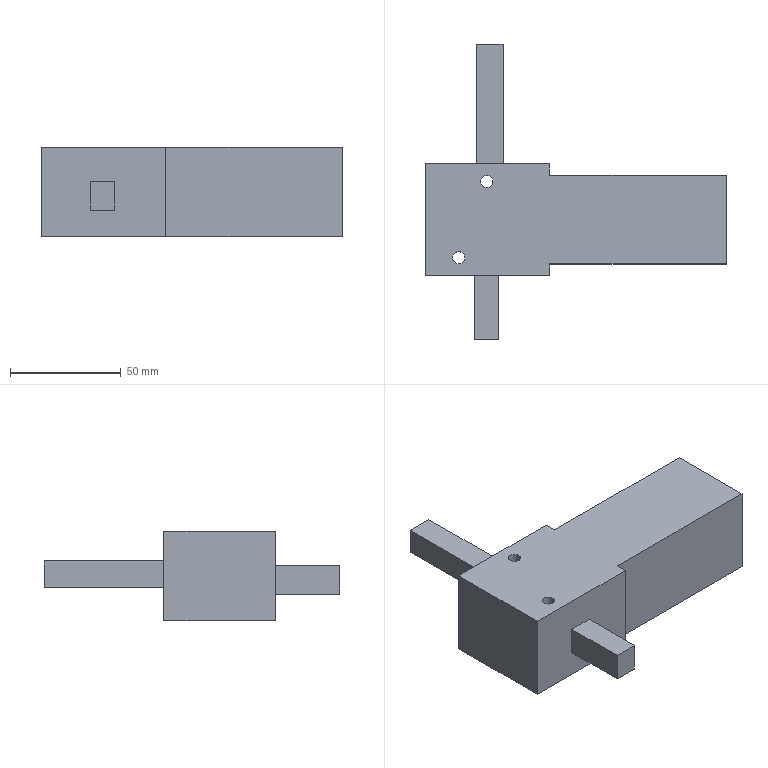Part | SolidWorks | features BaseBody 1 | 1 solid | 256 faces | box 135.9 x 133.4 x 40.4 mm | volume 252596 mm3 | plane 146 | spline 102 | cylinder 8 | commonest cylinder face diameters 5.5 x4 10 x4